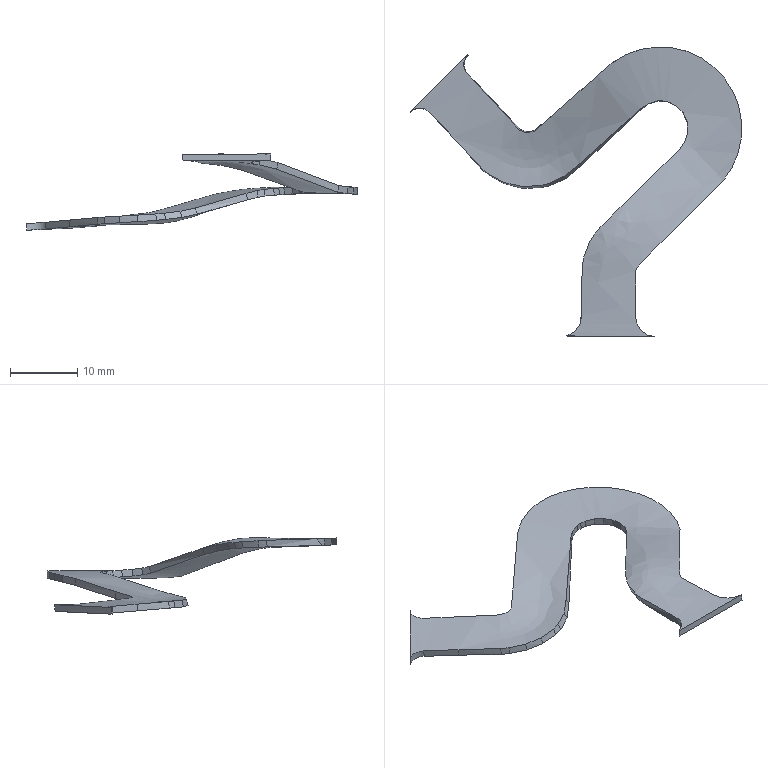Part | STEP file | gslz 2016.10.28-13_id1226_x_t | 1 solid | 70 faces | volume 746.006 mm3 | spline 70